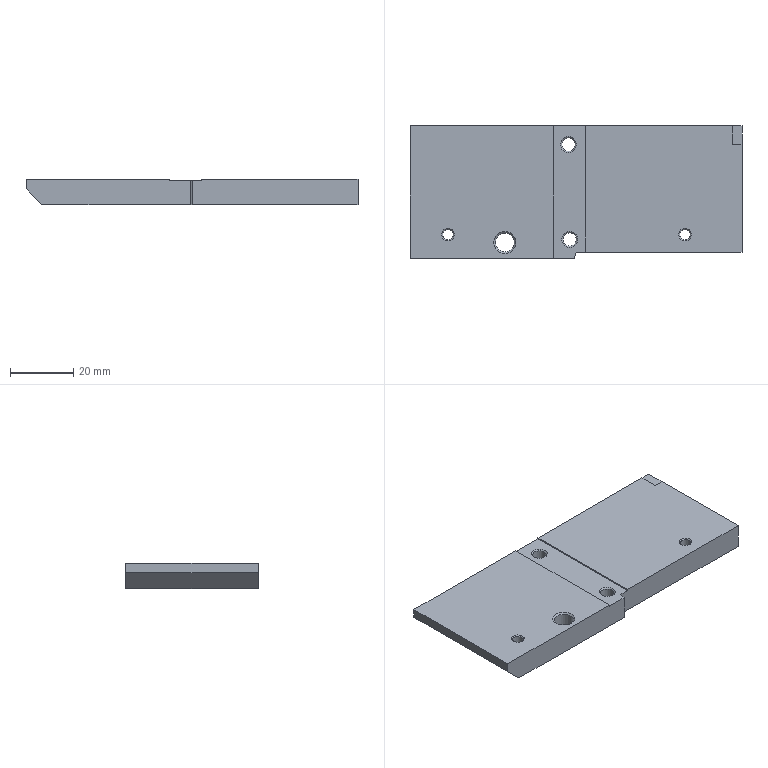Part | 2 solids | 51 faces | box 105 x 42 x 8 mm | volume 32745 mm3 | plane 21 | cone 20 | cylinder 10 | commonest cylinder face diameters 2.5 x4 4.2 x3 3.3 x2 6 x1
STEP:
#1=CARTESIAN_POINT('',(-22.5,21.,-6.2));
#2=VERTEX_POINT('',#1);
#3=CARTESIAN_POINT('',(-22.5,21.,-3.7));
#4=DIRECTION('',(0.,-1.,0.));
#5=DIRECTION('',(0.,0.,-1.));
#6=AXIS2_PLACEMENT_3D('',#3,#4,#5);
#7=CIRCLE('',#6,2.5);
#8=EDGE_CURVE('',#2,#2,#7,.T.);
#9=ORIENTED_EDGE('',*,*,#8,.T.);
#10=EDGE_LOOP('',(#9));
#11=FACE_BOUND('',#10,.T.);
#12=CARTESIAN_POINT('',(36.5,21.,-6.));
#13=VERTEX_POINT('',#12);
#14=CARTESIAN_POINT('',(36.5,21.,-4.5));
#15=DIRECTION('',(0.,-1.,0.));
#16=DIRECTION('',(0.,0.,-1.));
#17=AXIS2_PLACEMENT_3D('',#14,#15,#16);
#18=CIRCLE('',#17,1.5);
#19=EDGE_CURVE('',#13,#13,#18,.T.);
#20=ORIENTED_EDGE('',*,*,#19,.T.);
#21=EDGE_LOOP('',(#20));
#22=FACE_BOUND('',#21,.T.);
#23=CARTESIAN_POINT('',(8.5,21.,-6.));
#24=VERTEX_POINT('',#23);
#25=CARTESIAN_POINT('',(8.5,21.,-4.5));
#26=DIRECTION('',(0.,-1.,0.));
#27=DIRECTION('',(0.,0.,-1.));
#28=AXIS2_PLACEMENT_3D('',#25,#26,#27);
#29=CIRCLE('',#28,1.5);
#30=EDGE_CURVE('',#24,#24,#29,.T.);
#31=ORIENTED_EDGE('',*,*,#30,.T.);
#32=EDGE_LOOP('',(#31));
#33=FACE_BOUND('',#32,.T.);
#34=CARTESIAN_POINT('',(-36.5,21.,-5.2));
#35=VERTEX_POINT('',#34);
#36=CARTESIAN_POINT('',(-36.5,21.,-3.7));
#37=DIRECTION('',(0.,-1.,0.));
#38=DIRECTION('',(0.,0.,-1.));
#39=AXIS2_PLACEMENT_3D('',#36,#37,#38);
#40=CIRCLE('',#39,1.5);
#41=EDGE_CURVE('',#35,#35,#40,.T.);
#42=ORIENTED_EDGE('',*,*,#41,.T.);
#43=EDGE_LOOP('',(#42));
#44=FACE_BOUND('',#43,.T.);
#45=CARTESIAN_POINT('',(-44.5,21.,-5.2));
#46=VERTEX_POINT('',#45);
#47=CARTESIAN_POINT('',(-44.5,21.,-3.7));
#48=DIRECTION('',(0.,-1.,0.));
#49=DIRECTION('',(0.,0.,-1.));
#50=AXIS2_PLACEMENT_3D('',#47,#48,#49);
#51=CIRCLE('',#50,1.5);
#52=EDGE_CURVE('',#46,#46,#51,.T.);
#53=ORIENTED_EDGE('',*,*,#52,.T.);
#54=EDGE_LOOP('',(#53));
#55=FACE_BOUND('',#54,.T.);
#56=CARTESIAN_POINT('',(-47.5,21.,-8.));
#57=VERTEX_POINT('',#56);
#58=CARTESIAN_POINT('',(49.5,21.,-8.));
#59=VERTEX_POINT('',#58);
#60=CARTESIAN_POINT('',(-52.5,21.,-8.));
#61=DIRECTION('',(1.,0.,0.));
#62=VECTOR('',#61,1000.);
#63=LINE('',#60,#62);
#64=EDGE_CURVE('',#57,#59,#63,.T.);
#65=ORIENTED_EDGE('',*,*,#64,.F.);
#66=CARTESIAN_POINT('',(-52.5,21.,-3.));
#67=VERTEX_POINT('',#66);
#68=CARTESIAN_POINT('',(-47.5,21.,-8.));
#69=DIRECTION('',(-0.7071,0.,0.7071));
#70=VECTOR('',#69,1000.);
#71=LINE('',#68,#70);
#72=EDGE_CURVE('',#57,#67,#71,.T.);
#73=ORIENTED_EDGE('',*,*,#72,.T.);
#74=CARTESIAN_POINT('',(-52.5,21.,0.));
#75=VERTEX_POINT('',#74);
#76=CARTESIAN_POINT('',(-52.5,21.,-8.));
#77=DIRECTION('',(0.,0.,1.));
#78=VECTOR('',#77,1000.);
#79=LINE('',#76,#78);
#80=EDGE_CURVE('',#67,#75,#79,.T.);
#81=ORIENTED_EDGE('',*,*,#80,.T.);
#82=CARTESIAN_POINT('',(-7.,21.,0.));
#83=VERTEX_POINT('',#82);
#84=CARTESIAN_POINT('',(-52.5,21.,0.));
#85=DIRECTION('',(1.,0.,0.));
#86=VECTOR('',#85,1000.);
#87=LINE('',#84,#86);
#88=EDGE_CURVE('',#75,#83,#87,.T.);
#89=ORIENTED_EDGE('',*,*,#88,.T.);
#90=CARTESIAN_POINT('',(-7.,21.,-0.4));
#91=VERTEX_POINT('',#90);
#92=CARTESIAN_POINT('',(-7.,21.,-0.4));
#93=DIRECTION('',(0.,0.,1.));
#94=VECTOR('',#93,1000.);
#95=LINE('',#92,#94);
#96=EDGE_CURVE('',#91,#83,#95,.T.);
#97=ORIENTED_EDGE('',*,*,#96,.F.);
#98=CARTESIAN_POINT('',(3.,21.,-0.4));
#99=VERTEX_POINT('',#98);
#100=CARTESIAN_POINT('',(3.,21.,-0.4));
#101=DIRECTION('',(-1.,0.,0.));
#102=VECTOR('',#101,1000.);
#103=LINE('',#100,#102);
#104=EDGE_CURVE('',#99,#91,#103,.T.);
#105=ORIENTED_EDGE('',*,*,#104,.F.);
#106=CARTESIAN_POINT('',(3.,21.,0.));
#107=VERTEX_POINT('',#106);
#108=CARTESIAN_POINT('',(3.,21.,0.));
#109=DIRECTION('',(0.,0.,-1.));
#110=VECTOR('',#109,1000.);
#111=LINE('',#108,#110);
#112=EDGE_CURVE('',#107,#99,#111,.T.);
#113=ORIENTED_EDGE('',*,*,#112,.F.);
#114=CARTESIAN_POINT('',(49.5,21.,0.));
#115=VERTEX_POINT('',#114);
#116=CARTESIAN_POINT('',(-52.5,21.,0.));
#117=DIRECTION('',(1.,0.,0.));
#118=VECTOR('',#117,1000.);
#119=LINE('',#116,#118);
#120=EDGE_CURVE('',#107,#115,#119,.T.);
#121=ORIENTED_EDGE('',*,*,#120,.T.);
#122=CARTESIAN_POINT('',(49.5,21.,-8.));
#123=DIRECTION('',(0.,0.,1.));
#124=VECTOR('',#123,1000.);
#125=LINE('',#122,#124);
#126=EDGE_CURVE('',#59,#115,#125,.T.);
#127=ORIENTED_EDGE('',*,*,#126,.F.);
#128=EDGE_LOOP('',(#65,#73,#81,#89,#97,#105,#113,#121,#127));
#129=FACE_BOUND('',#128,.T.);
#130=CARTESIAN_POINT('',(-52.5,21.,-8.));
#131=DIRECTION('',(0.,-1.,0.));
#132=DIRECTION('',(0.,0.,1.));
#133=AXIS2_PLACEMENT_3D('',#130,#131,#132);
#134=PLANE('',#133);
#135=ADVANCED_FACE('',(#11,#22,#33,#44,#55,#129),#134,.F.);
#136=CARTESIAN_POINT('',(34.5,-11.5,0.));
#137=VERTEX_POINT('',#136);
#138=CARTESIAN_POINT('',(34.5,-13.5,0.));
#139=DIRECTION('',(0.,0.,-1.));
#140=DIRECTION('',(0.,1.,0.));
#141=AXIS2_PLACEMENT_3D('',#138,#139,#140);
#142=CIRCLE('',#141,2.);
#143=EDGE_CURVE('',#137,#137,#142,.T.);
#144=ORIENTED_EDGE('',*,*,#143,.T.);
#145=EDGE_LOOP('',(#144));
#146=FACE_BOUND('',#145,.T.);
#147=CARTESIAN_POINT('',(3.,-19.,0.));
#148=VERTEX_POINT('',#147);
#149=CARTESIAN_POINT('',(3.,-76.,0.));
#150=DIRECTION('',(0.,1.,0.));
#151=VECTOR('',#150,1000.);
#152=LINE('',#149,#151);
#153=EDGE_CURVE('',#148,#107,#152,.T.);
#154=ORIENTED_EDGE('',*,*,#153,.F.);
#155=CARTESIAN_POINT('',(52.5,-19.,0.));
#156=VERTEX_POINT('',#155);
#157=CARTESIAN_POINT('',(52.5,-19.,0.));
#158=DIRECTION('',(-1.,0.,0.));
#159=VECTOR('',#158,1000.);
#160=LINE('',#157,#159);
#161=EDGE_CURVE('',#156,#148,#160,.T.);
#162=ORIENTED_EDGE('',*,*,#161,.F.);
#163=CARTESIAN_POINT('',(52.5,15.,0.));
#164=VERTEX_POINT('',#163);
#165=CARTESIAN_POINT('',(52.5,15.,0.));
#166=DIRECTION('',(0.,-1.,0.));
#167=VECTOR('',#166,1000.);
#168=LINE('',#165,#167);
#169=EDGE_CURVE('',#164,#156,#168,.T.);
#170=ORIENTED_EDGE('',*,*,#169,.F.);
#171=CARTESIAN_POINT('',(49.5,15.,0.));
#172=VERTEX_POINT('',#171);
#173=CARTESIAN_POINT('',(49.5,15.,0.));
#174=DIRECTION('',(1.,0.,0.));
#175=VECTOR('',#174,1000.);
#176=LINE('',#173,#175);
#177=EDGE_CURVE('',#172,#164,#176,.T.);
#178=ORIENTED_EDGE('',*,*,#177,.F.);
#179=CARTESIAN_POINT('',(49.5,21.,0.));
#180=DIRECTION('',(0.,-1.,0.));
#181=VECTOR('',#180,1000.);
#182=LINE('',#179,#181);
#183=EDGE_CURVE('',#115,#172,#182,.T.);
#184=ORIENTED_EDGE('',*,*,#183,.F.);
#185=ORIENTED_EDGE('',*,*,#120,.F.);
#186=EDGE_LOOP('',(#154,#162,#170,#178,#184,#185));
#187=FACE_BOUND('',#186,.T.);
#188=CARTESIAN_POINT('',(-52.5,21.,0.));
#189=DIRECTION('',(0.,0.,-1.));
#190=DIRECTION('',(0.,-1.,0.));
#191=AXIS2_PLACEMENT_3D('',#188,#189,#190);
#192=PLANE('',#191);
#193=ADVANCED_FACE('',(#146,#187),#192,.F.);
#194=CARTESIAN_POINT('',(-52.5,-21.,-3.));
#195=VERTEX_POINT('',#194);
#196=CARTESIAN_POINT('',(-52.5,-21.,0.));
#197=VERTEX_POINT('',#196);
#198=CARTESIAN_POINT('',(-52.5,-21.,-8.));
#199=DIRECTION('',(0.,0.,1.));
#200=VECTOR('',#199,1000.);
#201=LINE('',#198,#200);
#202=EDGE_CURVE('',#195,#197,#201,.T.);
#203=ORIENTED_EDGE('',*,*,#202,.F.);
#204=CARTESIAN_POINT('',(-47.5,-21.,-8.));
#205=VERTEX_POINT('',#204);
#206=CARTESIAN_POINT('',(-47.5,-21.,-8.));
#207=DIRECTION('',(0.7071,0.,-0.7071));
#208=VECTOR('',#207,1000.);
#209=LINE('',#206,#208);
#210=EDGE_CURVE('',#195,#205,#209,.T.);
#211=ORIENTED_EDGE('',*,*,#210,.T.);
#212=CARTESIAN_POINT('',(-0.5,-21.,-8.));
#213=VERTEX_POINT('',#212);
#214=CARTESIAN_POINT('',(-0.5,-21.,-8.));
#215=DIRECTION('',(-1.,0.,0.));
#216=VECTOR('',#215,1000.);
#217=LINE('',#214,#216);
#218=EDGE_CURVE('',#213,#205,#217,.T.);
#219=ORIENTED_EDGE('',*,*,#218,.F.);
#220=CARTESIAN_POINT('',(-0.5,-21.,-0.4));
#221=VERTEX_POINT('',#220);
#222=CARTESIAN_POINT('',(-0.5,-21.,-8.));
#223=DIRECTION('',(0.,0.,1.));
#224=VECTOR('',#223,1000.);
#225=LINE('',#222,#224);
#226=EDGE_CURVE('',#213,#221,#225,.T.);
#227=ORIENTED_EDGE('',*,*,#226,.T.);
#228=CARTESIAN_POINT('',(-7.,-21.,-0.4));
#229=VERTEX_POINT('',#228);
#230=CARTESIAN_POINT('',(-0.5,-21.,-0.4));
#231=DIRECTION('',(-1.,0.,0.));
#232=VECTOR('',#231,1000.);
#233=LINE('',#230,#232);
#234=EDGE_CURVE('',#221,#229,#233,.T.);
#235=ORIENTED_EDGE('',*,*,#234,.T.);
#236=CARTESIAN_POINT('',(-7.,-21.,0.));
#237=VERTEX_POINT('',#236);
#238=CARTESIAN_POINT('',(-7.,-21.,-8.));
#239=DIRECTION('',(0.,0.,1.));
#240=VECTOR('',#239,1000.);
#241=LINE('',#238,#240);
#242=EDGE_CURVE('',#229,#237,#241,.T.);
#243=ORIENTED_EDGE('',*,*,#242,.T.);
#244=CARTESIAN_POINT('',(-0.5,-21.,0.));
#245=DIRECTION('',(-1.,0.,0.));
#246=VECTOR('',#245,1000.);
#247=LINE('',#244,#246);
#248=EDGE_CURVE('',#237,#197,#247,.T.);
#249=ORIENTED_EDGE('',*,*,#248,.T.);
#250=EDGE_LOOP('',(#203,#211,#219,#227,#235,#243,#249));
#251=FACE_BOUND('',#250,.T.);
#252=CARTESIAN_POINT('',(-0.5,-21.,-8.));
#253=DIRECTION('',(0.,1.,0.));
#254=DIRECTION('',(0.,0.,-1.));
#255=AXIS2_PLACEMENT_3D('',#252,#253,#254);
#256=PLANE('',#255);
#257=ADVANCED_FACE('',(#251),#256,.F.);
#258=ORIENTED_EDGE('',*,*,#80,.F.);
#259=CARTESIAN_POINT('',(-52.5,-21.,-3.));
#260=DIRECTION('',(0.,-1.,0.));
#261=VECTOR('',#260,1000.);
#262=LINE('',#259,#261);
#263=EDGE_CURVE('',#67,#195,#262,.T.);
#264=ORIENTED_EDGE('',*,*,#263,.T.);
#265=ORIENTED_EDGE('',*,*,#202,.T.);
#266=CARTESIAN_POINT('',(-52.5,-21.,0.));
#267=DIRECTION('',(0.,1.,0.));
#268=VECTOR('',#267,1000.);
#269=LINE('',#266,#268);
#270=EDGE_CURVE('',#197,#75,#269,.T.);
#271=ORIENTED_EDGE('',*,*,#270,.T.);
#272=EDGE_LOOP('',(#258,#264,#265,#271));
#273=FACE_BOUND('',#272,.T.);
#274=CARTESIAN_POINT('',(-52.5,-21.,-8.));
#275=DIRECTION('',(1.,0.,0.));
#276=DIRECTION('',(0.,1.,0.));
#277=AXIS2_PLACEMENT_3D('',#274,#275,#276);
#278=PLANE('',#277);
#279=ADVANCED_FACE('',(#273),#278,.F.);
#280=ORIENTED_EDGE('',*,*,#183,.T.);
#281=CARTESIAN_POINT('',(49.5,15.,-8.));
#282=VERTEX_POINT('',#281);
#283=CARTESIAN_POINT('',(49.5,15.,-8.));
#284=DIRECTION('',(0.,0.,1.));
#285=VECTOR('',#284,1000.);
#286=LINE('',#283,#285);
#287=EDGE_CURVE('',#282,#172,#286,.T.);
#288=ORIENTED_EDGE('',*,*,#287,.F.);
#289=CARTESIAN_POINT('',(49.5,21.,-8.));
#290=DIRECTION('',(0.,-1.,0.));
#291=VECTOR('',#290,1000.);
#292=LINE('',#289,#291);
#293=EDGE_CURVE('',#59,#282,#292,.T.);
#294=ORIENTED_EDGE('',*,*,#293,.F.);
#295=ORIENTED_EDGE('',*,*,#126,.T.);
#296=EDGE_LOOP('',(#280,#288,#294,#295));
#297=FACE_BOUND('',#296,.T.);
#298=CARTESIAN_POINT('',(49.5,21.,-8.));
#299=DIRECTION('',(-1.,0.,0.));
#300=DIRECTION('',(0.,-1.,0.));
#301=AXIS2_PLACEMENT_3D('',#298,#299,#300);
#302=PLANE('',#301);
#303=ADVANCED_FACE('',(#297),#302,.F.);
#304=ORIENTED_EDGE('',*,*,#177,.T.);
#305=CARTESIAN_POINT('',(52.5,15.,-8.));
#306=VERTEX_POINT('',#305);
#307=CARTESIAN_POINT('',(52.5,15.,-8.));
#308=DIRECTION('',(0.,0.,1.));
#309=VECTOR('',#308,1000.);
#310=LINE('',#307,#309);
#311=EDGE_CURVE('',#306,#164,#310,.T.);
#312=ORIENTED_EDGE('',*,*,#311,.F.);
#313=CARTESIAN_POINT('',(49.5,15.,-8.));
#314=DIRECTION('',(1.,0.,0.));
#315=VECTOR('',#314,1000.);
#316=LINE('',#313,#315);
#317=EDGE_CURVE('',#282,#306,#316,.T.);
#318=ORIENTED_EDGE('',*,*,#317,.F.);
#319=ORIENTED_EDGE('',*,*,#287,.T.);
#320=EDGE_LOOP('',(#304,#312,#318,#319));
#321=FACE_BOUND('',#320,.T.);
#322=CARTESIAN_POINT('',(49.5,15.,-8.));
#323=DIRECTION('',(0.,-1.,0.));
#324=DIRECTION('',(0.,0.,1.));
#325=AXIS2_PLACEMENT_3D('',#322,#323,#324);
#326=PLANE('',#325);
#327=ADVANCED_FACE('',(#321),#326,.F.);
#328=ORIENTED_EDGE('',*,*,#169,.T.);
#329=CARTESIAN_POINT('',(52.5,-19.,-8.));
#330=VERTEX_POINT('',#329);
#331=CARTESIAN_POINT('',(52.5,-19.,-8.));
#332=DIRECTION('',(0.,0.,1.));
#333=VECTOR('',#332,1000.);
#334=LINE('',#331,#333);
#335=EDGE_CURVE('',#330,#156,#334,.T.);
#336=ORIENTED_EDGE('',*,*,#335,.F.);
#337=CARTESIAN_POINT('',(52.5,15.,-8.));
#338=DIRECTION('',(0.,-1.,0.));
#339=VECTOR('',#338,1000.);
#340=LINE('',#337,#339);
#341=EDGE_CURVE('',#306,#330,#340,.T.);
#342=ORIENTED_EDGE('',*,*,#341,.F.);
#343=ORIENTED_EDGE('',*,*,#311,.T.);
#344=EDGE_LOOP('',(#328,#336,#342,#343));
#345=FACE_BOUND('',#344,.T.);
#346=CARTESIAN_POINT('',(52.5,15.,-8.));
#347=DIRECTION('',(-1.,0.,0.));
#348=DIRECTION('',(0.,-1.,0.));
#349=AXIS2_PLACEMENT_3D('',#346,#347,#348);
#350=PLANE('',#349);
#351=ADVANCED_FACE('',(#345),#350,.F.);
#352=CARTESIAN_POINT('',(3.,-19.,-0.4));
#353=VERTEX_POINT('',#352);
#354=CARTESIAN_POINT('',(3.,-19.,-8.));
#355=DIRECTION('',(0.,0.,-1.));
#356=VECTOR('',#355,1000.);
#357=LINE('',#354,#356);
#358=EDGE_CURVE('',#148,#353,#357,.T.);
#359=ORIENTED_EDGE('',*,*,#358,.T.);
#360=CARTESIAN_POINT('',(0.0359,-19.,-0.4));
#361=VERTEX_POINT('',#360);
#362=CARTESIAN_POINT('',(52.5,-19.,-0.4));
#363=DIRECTION('',(-1.,0.,0.));
#364=VECTOR('',#363,1000.);
#365=LINE('',#362,#364);
#366=EDGE_CURVE('',#353,#361,#365,.T.);
#367=ORIENTED_EDGE('',*,*,#366,.T.);
#368=CARTESIAN_POINT('',(0.0359,-19.,-8.));
#369=VERTEX_POINT('',#368);
#370=CARTESIAN_POINT('',(0.0359,-19.,-8.));
#371=DIRECTION('',(0.,0.,1.));
#372=VECTOR('',#371,1000.);
#373=LINE('',#370,#372);
#374=EDGE_CURVE('',#369,#361,#373,.T.);
#375=ORIENTED_EDGE('',*,*,#374,.F.);
#376=CARTESIAN_POINT('',(52.5,-19.,-8.));
#377=DIRECTION('',(-1.,0.,0.));
#378=VECTOR('',#377,1000.);
#379=LINE('',#376,#378);
#380=EDGE_CURVE('',#330,#369,#379,.T.);
#381=ORIENTED_EDGE('',*,*,#380,.F.);
#382=ORIENTED_EDGE('',*,*,#335,.T.);
#383=ORIENTED_EDGE('',*,*,#161,.T.);
#384=EDGE_LOOP('',(#359,#367,#375,#381,#382,#383));
#385=FACE_BOUND('',#384,.T.);
#386=CARTESIAN_POINT('',(52.5,-19.,-8.));
#387=DIRECTION('',(0.,1.,0.));
#388=DIRECTION('',(0.,0.,-1.));
#389=AXIS2_PLACEMENT_3D('',#386,#387,#388);
#390=PLANE('',#389);
#391=ADVANCED_FACE('',(#385),#390,.F.);
#392=ORIENTED_EDGE('',*,*,#374,.T.);
#393=CARTESIAN_POINT('',(0.0359,-19.,-0.4));
#394=DIRECTION('',(-0.2588,-0.9659,0.));
#395=VECTOR('',#394,1000.);
#396=LINE('',#393,#395);
#397=EDGE_CURVE('',#361,#221,#396,.T.);
#398=ORIENTED_EDGE('',*,*,#397,.T.);
#399=ORIENTED_EDGE('',*,*,#226,.F.);
#400=CARTESIAN_POINT('',(0.0359,-19.,-8.));
#401=DIRECTION('',(-0.2588,-0.9659,0.));
#402=VECTOR('',#401,1000.);
#403=LINE('',#400,#402);
#404=EDGE_CURVE('',#369,#213,#403,.T.);
#405=ORIENTED_EDGE('',*,*,#404,.F.);
#406=EDGE_LOOP('',(#392,#398,#399,#405));
#407=FACE_BOUND('',#406,.T.);
#408=CARTESIAN_POINT('',(0.0359,-19.,-8.));
#409=DIRECTION('',(-0.9659,0.2588,0.));
#410=DIRECTION('',(-0.2588,-0.9659,0.));
#411=AXIS2_PLACEMENT_3D('',#408,#409,#410);
#412=PLANE('',#411);
#413=ADVANCED_FACE('',(#407),#412,.F.);
#414=CARTESIAN_POINT('',(-22.5,-12.5,-8.));
#415=VERTEX_POINT('',#414);
#416=CARTESIAN_POINT('',(-22.5,-16.,-8.));
#417=DIRECTION('',(0.,0.,-1.));
#418=DIRECTION('',(0.,1.,0.));
#419=AXIS2_PLACEMENT_3D('',#416,#417,#418);
#420=CIRCLE('',#419,3.5);
#421=EDGE_CURVE('',#415,#415,#420,.T.);
#422=ORIENTED_EDGE('',*,*,#421,.F.);
#423=EDGE_LOOP('',(#422));
#424=FACE_BOUND('',#423,.T.);
#425=CARTESIAN_POINT('',(34.5,-11.5,-8.));
#426=VERTEX_POINT('',#425);
#427=CARTESIAN_POINT('',(34.5,-13.5,-8.));
#428=DIRECTION('',(0.,0.,-1.));
#429=DIRECTION('',(0.,1.,0.));
#430=AXIS2_PLACEMENT_3D('',#427,#428,#429);
#431=CIRCLE('',#430,2.);
#432=EDGE_CURVE('',#426,#426,#431,.T.);
#433=ORIENTED_EDGE('',*,*,#432,.F.);
#434=EDGE_LOOP('',(#433));
#435=FACE_BOUND('',#434,.T.);
#436=CARTESIAN_POINT('',(-40.5,-11.5,-8.));
#437=VERTEX_POINT('',#436);
#438=CARTESIAN_POINT('',(-40.5,-13.5,-8.));
#439=DIRECTION('',(0.,0.,-1.));
#440=DIRECTION('',(0.,1.,0.));
#441=AXIS2_PLACEMENT_3D('',#438,#439,#440);
#442=CIRCLE('',#441,2.);
#443=EDGE_CURVE('',#437,#437,#442,.T.);
#444=ORIENTED_EDGE('',*,*,#443,.F.);
#445=EDGE_LOOP('',(#444));
#446=FACE_BOUND('',#445,.T.);
#447=CARTESIAN_POINT('',(-2.,-12.5,-8.));
#448=VERTEX_POINT('',#447);
#449=CARTESIAN_POINT('',(-2.,-15.,-8.));
#450=DIRECTION('',(0.,0.,-1.));
#451=DIRECTION('',(0.,1.,0.));
#452=AXIS2_PLACEMENT_3D('',#449,#450,#451);
#453=CIRCLE('',#452,2.5);
#454=EDGE_CURVE('',#448,#448,#453,.T.);
#455=ORIENTED_EDGE('',*,*,#454,.F.);
#456=EDGE_LOOP('',(#455));
#457=FACE_BOUND('',#456,.T.);
#458=CARTESIAN_POINT('',(-2.382,17.498,-8.));
#459=VERTEX_POINT('',#458);
#460=CARTESIAN_POINT('',(-2.382,14.998,-8.));
#461=DIRECTION('',(0.,0.,-1.));
#462=DIRECTION('',(0.,1.,0.));
#463=AXIS2_PLACEMENT_3D('',#460,#461,#462);
#464=CIRCLE('',#463,2.5);
#465=EDGE_CURVE('',#459,#459,#464,.T.);
#466=ORIENTED_EDGE('',*,*,#465,.F.);
#467=EDGE_LOOP('',(#466));
#468=FACE_BOUND('',#467,.T.);
#469=ORIENTED_EDGE('',*,*,#218,.T.);
#470=CARTESIAN_POINT('',(-47.5,21.,-8.));
#471=DIRECTION('',(0.,1.,0.));
#472=VECTOR('',#471,1000.);
#473=LINE('',#470,#472);
#474=EDGE_CURVE('',#205,#57,#473,.T.);
#475=ORIENTED_EDGE('',*,*,#474,.T.);
#476=ORIENTED_EDGE('',*,*,#64,.T.);
#477=ORIENTED_EDGE('',*,*,#293,.T.);
#478=ORIENTED_EDGE('',*,*,#317,.T.);
#479=ORIENTED_EDGE('',*,*,#341,.T.);
#480=ORIENTED_EDGE('',*,*,#380,.T.);
#481=ORIENTED_EDGE('',*,*,#404,.T.);
#482=EDGE_LOOP('',(#469,#475,#476,#477,#478,#479,#480,#481));
#483=FACE_BOUND('',#482,.T.);
#484=CARTESIAN_POINT('',(-52.5,21.,-8.));
#485=DIRECTION('',(0.,0.,-1.));
#486=DIRECTION('',(0.,-1.,0.));
#487=AXIS2_PLACEMENT_3D('',#484,#485,#486);
#488=PLANE('',#487);
#489=ADVANCED_FACE('',(#424,#435,#446,#457,#468,#483),#488,.T.);
#490=CARTESIAN_POINT('',(-22.5,-12.5,0.));
#491=VERTEX_POINT('',#490);
#492=CARTESIAN_POINT('',(-22.5,-16.,0.));
#493=DIRECTION('',(0.,0.,-1.));
#494=DIRECTION('',(0.,1.,0.));
#495=AXIS2_PLACEMENT_3D('',#492,#493,#494);
#496=CIRCLE('',#495,3.5);
#497=EDGE_CURVE('',#491,#491,#496,.T.);
#498=ORIENTED_EDGE('',*,*,#497,.T.);
#499=EDGE_LOOP('',(#498));
#500=FACE_BOUND('',#499,.T.);
#501=CARTESIAN_POINT('',(-40.5,-11.5,0.));
#502=VERTEX_POINT('',#501);
#503=CARTESIAN_POINT('',(-40.5,-13.5,0.));
#504=DIRECTION('',(0.,0.,-1.));
#505=DIRECTION('',(0.,1.,0.));
#506=AXIS2_PLACEMENT_3D('',#503,#504,#505);
#507=CIRCLE('',#506,2.);
#508=EDGE_CURVE('',#502,#502,#507,.T.);
#509=ORIENTED_EDGE('',*,*,#508,.T.);
#510=EDGE_LOOP('',(#509));
#511=FACE_BOUND('',#510,.T.);
#512=ORIENTED_EDGE('',*,*,#248,.F.);
#513=CARTESIAN_POINT('',(-7.,-76.,0.));
#514=DIRECTION('',(0.,1.,0.));
#515=VECTOR('',#514,1000.);
#516=LINE('',#513,#515);
#517=EDGE_CURVE('',#237,#83,#516,.T.);
#518=ORIENTED_EDGE('',*,*,#517,.T.);
#519=ORIENTED_EDGE('',*,*,#88,.F.);
#520=ORIENTED_EDGE('',*,*,#270,.F.);
#521=EDGE_LOOP('',(#512,#518,#519,#520));
#522=FACE_BOUND('',#521,.T.);
#523=CARTESIAN_POINT('',(-52.5,21.,0.));
#524=DIRECTION('',(0.,0.,-1.));
#525=DIRECTION('',(0.,-1.,0.));
#526=AXIS2_PLACEMENT_3D('',#523,#524,#525);
#527=PLANE('',#526);
#528=ADVANCED_FACE('',(#500,#511,#522),#527,.F.);
#529=CARTESIAN_POINT('',(-7.,-76.,-0.4));
#530=DIRECTION('',(0.,-1.,0.));
#531=VECTOR('',#530,1000.);
#532=LINE('',#529,#531);
#533=EDGE_CURVE('',#91,#229,#532,.T.);
#534=ORIENTED_EDGE('',*,*,#533,.F.);
#535=ORIENTED_EDGE('',*,*,#96,.T.);
#536=ORIENTED_EDGE('',*,*,#517,.F.);
#537=ORIENTED_EDGE('',*,*,#242,.F.);
#538=EDGE_LOOP('',(#534,#535,#536,#537));
#539=FACE_BOUND('',#538,.T.);
#540=CARTESIAN_POINT('',(-7.,-76.,-0.4));
#541=DIRECTION('',(-1.,0.,0.));
#542=DIRECTION('',(0.,-1.,0.));
#543=AXIS2_PLACEMENT_3D('',#540,#541,#542);
#544=PLANE('',#543);
#545=ADVANCED_FACE('',(#539),#544,.F.);
#546=CARTESIAN_POINT('',(-2.,-12.5,-0.4));
#547=VERTEX_POINT('',#546);
#548=CARTESIAN_POINT('',(-2.,-15.,-0.4));
#549=DIRECTION('',(0.,0.,-1.));
#550=DIRECTION('',(0.,1.,0.));
#551=AXIS2_PLACEMENT_3D('',#548,#549,#550);
#552=CIRCLE('',#551,2.5);
#553=EDGE_CURVE('',#547,#547,#552,.T.);
#554=ORIENTED_EDGE('',*,*,#553,.T.);
#555=EDGE_LOOP('',(#554));
#556=FACE_BOUND('',#555,.T.);
#557=CARTESIAN_POINT('',(-2.382,17.498,-0.4));
#558=VERTEX_POINT('',#557);
#559=CARTESIAN_POINT('',(-2.382,14.998,-0.4));
#560=DIRECTION('',(0.,0.,-1.));
#561=DIRECTION('',(0.,1.,0.));
#562=AXIS2_PLACEMENT_3D('',#559,#560,#561);
#563=CIRCLE('',#562,2.5);
#564=EDGE_CURVE('',#558,#558,#563,.T.);
#565=ORIENTED_EDGE('',*,*,#564,.T.);
#566=EDGE_LOOP('',(#565));
#567=FACE_BOUND('',#566,.T.);
#568=ORIENTED_EDGE('',*,*,#397,.F.);
#569=ORIENTED_EDGE('',*,*,#366,.F.);
#570=CARTESIAN_POINT('',(3.,-76.,-0.4));
#571=DIRECTION('',(0.,-1.,0.));
#572=VECTOR('',#571,1000.);
#573=LINE('',#570,#572);
#574=EDGE_CURVE('',#99,#353,#573,.T.);
#575=ORIENTED_EDGE('',*,*,#574,.F.);
#576=ORIENTED_EDGE('',*,*,#104,.T.);
#577=ORIENTED_EDGE('',*,*,#533,.T.);
#578=ORIENTED_EDGE('',*,*,#234,.F.);
#579=EDGE_LOOP('',(#568,#569,#575,#576,#577,#578));
#580=FACE_BOUND('',#579,.T.);
#581=CARTESIAN_POINT('',(3.,-76.,-0.4));
#582=DIRECTION('',(0.,0.,-1.));
#583=DIRECTION('',(0.,-1.,0.));
#584=AXIS2_PLACEMENT_3D('',#581,#582,#583);
#585=PLANE('',#584);
#586=ADVANCED_FACE('',(#556,#567,#580),#585,.F.);
#587=ORIENTED_EDGE('',*,*,#153,.T.);
#588=ORIENTED_EDGE('',*,*,#112,.T.);
#589=ORIENTED_EDGE('',*,*,#574,.T.);
#590=ORIENTED_EDGE('',*,*,#358,.F.);
#591=EDGE_LOOP('',(#587,#588,#589,#590));
#592=FACE_BOUND('',#591,.T.);
#593=CARTESIAN_POINT('',(3.,-76.,0.));
#594=DIRECTION('',(1.,0.,0.));
#595=DIRECTION('',(0.,1.,0.));
#596=AXIS2_PLACEMENT_3D('',#593,#594,#595);
#597=PLANE('',#596);
#598=ADVANCED_FACE('',(#592),#597,.F.);
#599=CARTESIAN_POINT('',(-2.382,17.098,-7.6));
#600=VERTEX_POINT('',#599);
#601=CARTESIAN_POINT('',(-2.382,14.998,-7.6));
#602=DIRECTION('',(0.,0.,-1.));
#603=DIRECTION('',(0.,1.,0.));
#604=AXIS2_PLACEMENT_3D('',#601,#602,#603);
#605=CIRCLE('',#604,2.1);
#606=EDGE_CURVE('',#600,#600,#605,.T.);
#607=ORIENTED_EDGE('',*,*,#606,.T.);
#608=EDGE_LOOP('',(#607));
#609=FACE_BOUND('',#608,.T.);
#610=CARTESIAN_POINT('',(-2.382,12.898,-0.8));
#611=VERTEX_POINT('',#610);
#612=CARTESIAN_POINT('',(-2.382,14.998,-0.8));
#613=DIRECTION('',(0.,0.,1.));
#614=DIRECTION('',(0.,-1.,0.));
#615=AXIS2_PLACEMENT_3D('',#612,#613,#614);
#616=CIRCLE('',#615,2.1);
#617=EDGE_CURVE('',#611,#611,#616,.T.);
#618=ORIENTED_EDGE('',*,*,#617,.T.);
#619=EDGE_LOOP('',(#618));
#620=FACE_BOUND('',#619,.T.);
#621=CARTESIAN_POINT('',(-2.382,14.998,0.));
#622=DIRECTION('',(0.,0.,-1.));
#623=DIRECTION('',(0.,-1.,0.));
#624=AXIS2_PLACEMENT_3D('',#621,#622,#623);
#625=CYLINDRICAL_SURFACE('',#624,2.1);
#626=ADVANCED_FACE('',(#609,#620),#625,.F.);
#627=ORIENTED_EDGE('',*,*,#564,.F.);
#628=EDGE_LOOP('',(#627));
#629=FACE_BOUND('',#628,.T.);
#630=ORIENTED_EDGE('',*,*,#617,.F.);
#631=EDGE_LOOP('',(#630));
#632=FACE_BOUND('',#631,.T.);
#633=CARTESIAN_POINT('',(-2.382,14.998,-2.9));
#634=DIRECTION('',(0.,0.,1.));
#635=DIRECTION('',(1.,0.,0.));
#636=AXIS2_PLACEMENT_3D('',#633,#634,#635);
#637=CONICAL_SURFACE('',#636,0.,0.7854);
#638=ADVANCED_FACE('',(#629,#632),#637,.F.);
#639=ORIENTED_EDGE('',*,*,#465,.T.);
#640=EDGE_LOOP('',(#639));
#641=FACE_BOUND('',#640,.T.);
#642=ORIENTED_EDGE('',*,*,#606,.F.);
#643=EDGE_LOOP('',(#642));
#644=FACE_BOUND('',#643,.T.);
#645=CARTESIAN_POINT('',(-2.382,14.998,-5.5));
#646=DIRECTION('',(0.,0.,-1.));
#647=DIRECTION('',(-1.,0.,0.));
#648=AXIS2_PLACEMENT_3D('',#645,#646,#647);
#649=CONICAL_SURFACE('',#648,0.,0.7854);
#650=ADVANCED_FACE('',(#641,#644),#649,.F.);
#651=CARTESIAN_POINT('',(-2.,-12.9,-7.6));
#652=VERTEX_POINT('',#651);
#653=CARTESIAN_POINT('',(-2.,-15.,-7.6));
#654=DIRECTION('',(0.,0.,-1.));
#655=DIRECTION('',(0.,1.,0.));
#656=AXIS2_PLACEMENT_3D('',#653,#654,#655);
#657=CIRCLE('',#656,2.1);
#658=EDGE_CURVE('',#652,#652,#657,.T.);
#659=ORIENTED_EDGE('',*,*,#658,.T.);
#660=EDGE_LOOP('',(#659));
#661=FACE_BOUND('',#660,.T.);
#662=CARTESIAN_POINT('',(-2.,-17.1,-0.8));
#663=VERTEX_POINT('',#662);
#664=CARTESIAN_POINT('',(-2.,-15.,-0.8));
#665=DIRECTION('',(0.,0.,1.));
#666=DIRECTION('',(0.,-1.,0.));
#667=AXIS2_PLACEMENT_3D('',#664,#665,#666);
#668=CIRCLE('',#667,2.1);
#669=EDGE_CURVE('',#663,#663,#668,.T.);
#670=ORIENTED_EDGE('',*,*,#669,.T.);
#671=EDGE_LOOP('',(#670));
#672=FACE_BOUND('',#671,.T.);
#673=CARTESIAN_POINT('',(-2.,-15.,0.));
#674=DIRECTION('',(0.,0.,-1.));
#675=DIRECTION('',(0.,-1.,0.));
#676=AXIS2_PLACEMENT_3D('',#673,#674,#675);
#677=CYLINDRICAL_SURFACE('',#676,2.1);
#678=ADVANCED_FACE('',(#661,#672),#677,.F.);
#679=ORIENTED_EDGE('',*,*,#553,.F.);
#680=EDGE_LOOP('',(#679));
#681=FACE_BOUND('',#680,.T.);
#682=ORIENTED_EDGE('',*,*,#669,.F.);
#683=EDGE_LOOP('',(#682));
#684=FACE_BOUND('',#683,.T.);
#685=CARTESIAN_POINT('',(-2.,-15.,-2.9));
#686=DIRECTION('',(0.,0.,1.));
#687=DIRECTION('',(1.,0.,0.));
#688=AXIS2_PLACEMENT_3D('',#685,#686,#687);
#689=CONICAL_SURFACE('',#688,0.,0.7854);
#690=ADVANCED_FACE('',(#681,#684),#689,.F.);
#691=ORIENTED_EDGE('',*,*,#454,.T.);
#692=EDGE_LOOP('',(#691));
#693=FACE_BOUND('',#692,.T.);
#694=ORIENTED_EDGE('',*,*,#658,.F.);
#695=EDGE_LOOP('',(#694));
#696=FACE_BOUND('',#695,.T.);
#697=CARTESIAN_POINT('',(-2.,-15.,-5.5));
#698=DIRECTION('',(0.,0.,-1.));
#699=DIRECTION('',(-1.,0.,0.));
#700=AXIS2_PLACEMENT_3D('',#697,#698,#699);
#701=CONICAL_SURFACE('',#700,0.,0.7854);
#702=ADVANCED_FACE('',(#693,#696),#701,.F.);
#703=CARTESIAN_POINT('',(-40.5,-11.85,-7.65));
#704=VERTEX_POINT('',#703);
#705=CARTESIAN_POINT('',(-40.5,-13.5,-7.65));
#706=DIRECTION('',(0.,0.,-1.));
#707=DIRECTION('',(0.,1.,0.));
#708=AXIS2_PLACEMENT_3D('',#705,#706,#707);
#709=CIRCLE('',#708,1.65);
#710=EDGE_CURVE('',#704,#704,#709,.T.);
#711=ORIENTED_EDGE('',*,*,#710,.T.);
#712=EDGE_LOOP('',(#711));
#713=FACE_BOUND('',#712,.T.);
#714=CARTESIAN_POINT('',(-40.5,-15.15,-0.35));
#715=VERTEX_POINT('',#714);
#716=CARTESIAN_POINT('',(-40.5,-13.5,-0.35));
#717=DIRECTION('',(0.,0.,1.));
#718=DIRECTION('',(0.,-1.,0.));
#719=AXIS2_PLACEMENT_3D('',#716,#717,#718);
#720=CIRCLE('',#719,1.65);
#721=EDGE_CURVE('',#715,#715,#720,.T.);
#722=ORIENTED_EDGE('',*,*,#721,.T.);
#723=EDGE_LOOP('',(#722));
#724=FACE_BOUND('',#723,.T.);
#725=CARTESIAN_POINT('',(-40.5,-13.5,0.));
#726=DIRECTION('',(0.,0.,-1.));
#727=DIRECTION('',(0.,-1.,0.));
#728=AXIS2_PLACEMENT_3D('',#725,#726,#727);
#729=CYLINDRICAL_SURFACE('',#728,1.65);
#730=ADVANCED_FACE('',(#713,#724),#729,.F.);
#731=ORIENTED_EDGE('',*,*,#508,.F.);
#732=EDGE_LOOP('',(#731));
#733=FACE_BOUND('',#732,.T.);
#734=ORIENTED_EDGE('',*,*,#721,.F.);
#735=EDGE_LOOP('',(#734));
#736=FACE_BOUND('',#735,.T.);
#737=CARTESIAN_POINT('',(-40.5,-13.5,-2.));
#738=DIRECTION('',(0.,0.,1.));
#739=DIRECTION('',(1.,0.,0.));
#740=AXIS2_PLACEMENT_3D('',#737,#738,#739);
#741=CONICAL_SURFACE('',#740,0.,0.7854);
#742=ADVANCED_FACE('',(#733,#736),#741,.F.);
#743=ORIENTED_EDGE('',*,*,#443,.T.);
#744=EDGE_LOOP('',(#743));
#745=FACE_BOUND('',#744,.T.);
#746=ORIENTED_EDGE('',*,*,#710,.F.);
#747=EDGE_LOOP('',(#746));
#748=FACE_BOUND('',#747,.T.);
#749=CARTESIAN_POINT('',(-40.5,-13.5,-6.));
#750=DIRECTION('',(0.,0.,-1.));
#751=DIRECTION('',(-1.,0.,0.));
#752=AXIS2_PLACEMENT_3D('',#749,#750,#751);
#753=CONICAL_SURFACE('',#752,0.,0.7854);
#754=ADVANCED_FACE('',(#745,#748),#753,.F.);
#755=CARTESIAN_POINT('',(34.5,-11.85,-7.65));
#756=VERTEX_POINT('',#755);
#757=CARTESIAN_POINT('',(34.5,-13.5,-7.65));
#758=DIRECTION('',(0.,0.,-1.));
#759=DIRECTION('',(0.,1.,0.));
#760=AXIS2_PLACEMENT_3D('',#757,#758,#759);
#761=CIRCLE('',#760,1.65);
#762=EDGE_CURVE('',#756,#756,#761,.T.);
#763=ORIENTED_EDGE('',*,*,#762,.T.);
#764=EDGE_LOOP('',(#763));
#765=FACE_BOUND('',#764,.T.);
#766=CARTESIAN_POINT('',(34.5,-15.15,-0.35));
#767=VERTEX_POINT('',#766);
#768=CARTESIAN_POINT('',(34.5,-13.5,-0.35));
#769=DIRECTION('',(0.,0.,1.));
#770=DIRECTION('',(0.,-1.,0.));
#771=AXIS2_PLACEMENT_3D('',#768,#769,#770);
#772=CIRCLE('',#771,1.65);
#773=EDGE_CURVE('',#767,#767,#772,.T.);
#774=ORIENTED_EDGE('',*,*,#773,.T.);
#775=EDGE_LOOP('',(#774));
#776=FACE_BOUND('',#775,.T.);
#777=CARTESIAN_POINT('',(34.5,-13.5,0.));
#778=DIRECTION('',(0.,0.,-1.));
#779=DIRECTION('',(0.,-1.,0.));
#780=AXIS2_PLACEMENT_3D('',#777,#778,#779);
#781=CYLINDRICAL_SURFACE('',#780,1.65);
#782=ADVANCED_FACE('',(#765,#776),#781,.F.);
#783=ORIENTED_EDGE('',*,*,#143,.F.);
#784=EDGE_LOOP('',(#783));
#785=FACE_BOUND('',#784,.T.);
#786=ORIENTED_EDGE('',*,*,#773,.F.);
#787=EDGE_LOOP('',(#786));
#788=FACE_BOUND('',#787,.T.);
#789=CARTESIAN_POINT('',(34.5,-13.5,-2.));
#790=DIRECTION('',(0.,0.,1.));
#791=DIRECTION('',(1.,0.,0.));
#792=AXIS2_PLACEMENT_3D('',#789,#790,#791);
#793=CONICAL_SURFACE('',#792,0.,0.7854);
#794=ADVANCED_FACE('',(#785,#788),#793,.F.);
#795=ORIENTED_EDGE('',*,*,#432,.T.);
#796=EDGE_LOOP('',(#795));
#797=FACE_BOUND('',#796,.T.);
#798=ORIENTED_EDGE('',*,*,#762,.F.);
#799=EDGE_LOOP('',(#798));
#800=FACE_BOUND('',#799,.T.);
#801=CARTESIAN_POINT('',(34.5,-13.5,-6.));
#802=DIRECTION('',(0.,0.,-1.));
#803=DIRECTION('',(-1.,0.,0.));
#804=AXIS2_PLACEMENT_3D('',#801,#802,#803);
#805=CONICAL_SURFACE('',#804,0.,0.7854);
#806=ADVANCED_FACE('',(#797,#800),#805,.F.);
#807=CARTESIAN_POINT('',(-22.5,-13.,-7.5));
#808=VERTEX_POINT('',#807);
#809=CARTESIAN_POINT('',(-22.5,-16.,-7.5));
#810=DIRECTION('',(0.,0.,-1.));
#811=DIRECTION('',(0.,1.,0.));
#812=AXIS2_PLACEMENT_3D('',#809,#810,#811);
#813=CIRCLE('',#812,3.);
#814=EDGE_CURVE('',#808,#808,#813,.T.);
#815=ORIENTED_EDGE('',*,*,#814,.T.);
#816=EDGE_LOOP('',(#815));
#817=FACE_BOUND('',#816,.T.);
#818=CARTESIAN_POINT('',(-22.5,-19.,-0.5));
#819=VERTEX_POINT('',#818);
#820=CARTESIAN_POINT('',(-22.5,-16.,-0.5));
#821=DIRECTION('',(0.,0.,1.));
#822=DIRECTION('',(0.,-1.,0.));
#823=AXIS2_PLACEMENT_3D('',#820,#821,#822);
#824=CIRCLE('',#823,3.);
#825=EDGE_CURVE('',#819,#819,#824,.T.);
#826=ORIENTED_EDGE('',*,*,#825,.T.);
#827=EDGE_LOOP('',(#826));
#828=FACE_BOUND('',#827,.T.);
#829=CARTESIAN_POINT('',(-22.5,-16.,0.));
#830=DIRECTION('',(0.,0.,-1.));
#831=DIRECTION('',(0.,-1.,0.));
#832=AXIS2_PLACEMENT_3D('',#829,#830,#831);
#833=CYLINDRICAL_SURFACE('',#832,3.);
#834=ADVANCED_FACE('',(#817,#828),#833,.F.);
#835=ORIENTED_EDGE('',*,*,#497,.F.);
#836=EDGE_LOOP('',(#835));
#837=FACE_BOUND('',#836,.T.);
#838=ORIENTED_EDGE('',*,*,#825,.F.);
#839=EDGE_LOOP('',(#838));
#840=FACE_BOUND('',#839,.T.);
#841=CARTESIAN_POINT('',(-22.5,-16.,-3.5));
#842=DIRECTION('',(0.,0.,1.));
#843=DIRECTION('',(1.,0.,0.));
#844=AXIS2_PLACEMENT_3D('',#841,#842,#843);
#845=CONICAL_SURFACE('',#844,0.,0.7854);
#846=ADVANCED_FACE('',(#837,#840),#845,.F.);
#847=ORIENTED_EDGE('',*,*,#421,.T.);
#848=EDGE_LOOP('',(#847));
#849=FACE_BOUND('',#848,.T.);
#850=ORIENTED_EDGE('',*,*,#814,.F.);
#851=EDGE_LOOP('',(#850));
#852=FACE_BOUND('',#851,.T.);
#853=CARTESIAN_POINT('',(-22.5,-16.,-4.5));
#854=DIRECTION('',(0.,0.,-1.));
#855=DIRECTION('',(-1.,0.,0.));
#856=AXIS2_PLACEMENT_3D('',#853,#854,#855);
#857=CONICAL_SURFACE('',#856,0.,0.7854);
#858=ADVANCED_FACE('',(#849,#852),#857,.F.);
#859=ORIENTED_EDGE('',*,*,#210,.F.);
#860=ORIENTED_EDGE('',*,*,#263,.F.);
#861=ORIENTED_EDGE('',*,*,#72,.F.);
#862=ORIENTED_EDGE('',*,*,#474,.F.);
#863=EDGE_LOOP('',(#859,#860,#861,#862));
#864=FACE_BOUND('',#863,.T.);
#865=CARTESIAN_POINT('',(-47.5,21.,-8.));
#866=DIRECTION('',(-0.7071,0.,-0.7071));
#867=DIRECTION('',(0.,1.,0.));
#868=AXIS2_PLACEMENT_3D('',#865,#866,#867);
#869=PLANE('',#868);
#870=ADVANCED_FACE('',(#864),#869,.T.);
#871=ORIENTED_EDGE('',*,*,#52,.F.);
#872=EDGE_LOOP('',(#871));
#873=FACE_BOUND('',#872,.T.);
#874=CARTESIAN_POINT('',(-44.5,20.75,-2.45));
#875=VERTEX_POINT('',#874);
#876=CARTESIAN_POINT('',(-44.5,20.75,-3.7));
#877=DIRECTION('',(0.,1.,0.));
#878=DIRECTION('',(0.,0.,1.));
#879=AXIS2_PLACEMENT_3D('',#876,#877,#878);
#880=CIRCLE('',#879,1.25);
#881=EDGE_CURVE('',#875,#875,#880,.T.);
#882=ORIENTED_EDGE('',*,*,#881,.F.);
#883=EDGE_LOOP('',(#882));
#884=FACE_BOUND('',#883,.T.);
#885=CARTESIAN_POINT('',(-44.5,19.5,-3.7));
#886=DIRECTION('',(0.,1.,0.));
#887=DIRECTION('',(0.,0.,-1.));
#888=AXIS2_PLACEMENT_3D('',#885,#886,#887);
#889=CONICAL_SURFACE('',#888,0.,0.7854);
#890=ADVANCED_FACE('',(#873,#884),#889,.F.);
#891=CARTESIAN_POINT('',(-44.5,9.,-4.95));
#892=VERTEX_POINT('',#891);
#893=CARTESIAN_POINT('',(-44.5,9.,-3.7));
#894=DIRECTION('',(0.,1.,0.));
#895=DIRECTION('',(0.,0.,-1.));
#896=AXIS2_PLACEMENT_3D('',#893,#894,#895);
#897=CIRCLE('',#896,1.25);
#898=EDGE_CURVE('',#892,#892,#897,.T.);
#899=ORIENTED_EDGE('',*,*,#898,.T.);
#900=EDGE_LOOP('',(#899));
#901=FACE_BOUND('',#900,.T.);
#902=CARTESIAN_POINT('',(-44.5,8.249,-3.7));
#903=VERTEX_POINT('',#902);
#904=VERTEX_LOOP('',#903);
#905=FACE_BOUND('',#904,.T.);
#906=CARTESIAN_POINT('',(-44.5,9.,-3.7));
#907=DIRECTION('',(0.,1.,0.));
#908=DIRECTION('',(0.,0.,-1.));
#909=AXIS2_PLACEMENT_3D('',#906,#907,#908);
#910=CONICAL_SURFACE('',#909,1.25,1.03);
#911=ADVANCED_FACE('',(#901,#905),#910,.F.);
#912=ORIENTED_EDGE('',*,*,#881,.T.);
#913=EDGE_LOOP('',(#912));
#914=FACE_BOUND('',#913,.T.);
#915=ORIENTED_EDGE('',*,*,#898,.F.);
#916=EDGE_LOOP('',(#915));
#917=FACE_BOUND('',#916,.T.);
#918=CARTESIAN_POINT('',(-44.5,21.,-3.7));
#919=DIRECTION('',(0.,-1.,0.));
#920=DIRECTION('',(0.,0.,1.));
#921=AXIS2_PLACEMENT_3D('',#918,#919,#920);
#922=CYLINDRICAL_SURFACE('',#921,1.25);
#923=ADVANCED_FACE('',(#914,#917),#922,.F.);
#924=ORIENTED_EDGE('',*,*,#41,.F.);
#925=EDGE_LOOP('',(#924));
#926=FACE_BOUND('',#925,.T.);
#927=CARTESIAN_POINT('',(-36.5,20.75,-2.45));
#928=VERTEX_POINT('',#927);
#929=CARTESIAN_POINT('',(-36.5,20.75,-3.7));
#930=DIRECTION('',(0.,1.,0.));
#931=DIRECTION('',(0.,0.,1.));
#932=AXIS2_PLACEMENT_3D('',#929,#930,#931);
#933=CIRCLE('',#932,1.25);
#934=EDGE_CURVE('',#928,#928,#933,.T.);
#935=ORIENTED_EDGE('',*,*,#934,.F.);
#936=EDGE_LOOP('',(#935));
#937=FACE_BOUND('',#936,.T.);
#938=CARTESIAN_POINT('',(-36.5,19.5,-3.7));
#939=DIRECTION('',(0.,1.,0.));
#940=DIRECTION('',(0.,0.,-1.));
#941=AXIS2_PLACEMENT_3D('',#938,#939,#940);
#942=CONICAL_SURFACE('',#941,0.,0.7854);
#943=ADVANCED_FACE('',(#926,#937),#942,.F.);
#944=CARTESIAN_POINT('',(-36.5,9.,-4.95));
#945=VERTEX_POINT('',#944);
#946=CARTESIAN_POINT('',(-36.5,9.,-3.7));
#947=DIRECTION('',(0.,1.,0.));
#948=DIRECTION('',(0.,0.,-1.));
#949=AXIS2_PLACEMENT_3D('',#946,#947,#948);
#950=CIRCLE('',#949,1.25);
#951=EDGE_CURVE('',#945,#945,#950,.T.);
#952=ORIENTED_EDGE('',*,*,#951,.T.);
#953=EDGE_LOOP('',(#952));
#954=FACE_BOUND('',#953,.T.);
#955=CARTESIAN_POINT('',(-36.5,8.249,-3.7));
#956=VERTEX_POINT('',#955);
#957=VERTEX_LOOP('',#956);
#958=FACE_BOUND('',#957,.T.);
#959=CARTESIAN_POINT('',(-36.5,9.,-3.7));
#960=DIRECTION('',(0.,1.,0.));
#961=DIRECTION('',(0.,0.,-1.));
#962=AXIS2_PLACEMENT_3D('',#959,#960,#961);
#963=CONICAL_SURFACE('',#962,1.25,1.03);
#964=ADVANCED_FACE('',(#954,#958),#963,.F.);
#965=ORIENTED_EDGE('',*,*,#934,.T.);
#966=EDGE_LOOP('',(#965));
#967=FACE_BOUND('',#966,.T.);
#968=ORIENTED_EDGE('',*,*,#951,.F.);
#969=EDGE_LOOP('',(#968));
#970=FACE_BOUND('',#969,.T.);
#971=CARTESIAN_POINT('',(-36.5,21.,-3.7));
#972=DIRECTION('',(0.,-1.,0.));
#973=DIRECTION('',(0.,0.,1.));
#974=AXIS2_PLACEMENT_3D('',#971,#972,#973);
#975=CYLINDRICAL_SURFACE('',#974,1.25);
#976=ADVANCED_FACE('',(#967,#970),#975,.F.);
#977=ORIENTED_EDGE('',*,*,#30,.F.);
#978=EDGE_LOOP('',(#977));
#979=FACE_BOUND('',#978,.T.);
#980=CARTESIAN_POINT('',(8.5,20.75,-3.25));
#981=VERTEX_POINT('',#980);
#982=CARTESIAN_POINT('',(8.5,20.75,-4.5));
#983=DIRECTION('',(0.,1.,0.));
#984=DIRECTION('',(0.,0.,1.));
#985=AXIS2_PLACEMENT_3D('',#982,#983,#984);
#986=CIRCLE('',#985,1.25);
#987=EDGE_CURVE('',#981,#981,#986,.T.);
#988=ORIENTED_EDGE('',*,*,#987,.F.);
#989=EDGE_LOOP('',(#988));
#990=FACE_BOUND('',#989,.T.);
#991=CARTESIAN_POINT('',(8.5,19.5,-4.5));
#992=DIRECTION('',(0.,1.,0.));
#993=DIRECTION('',(0.,0.,-1.));
#994=AXIS2_PLACEMENT_3D('',#991,#992,#993);
#995=CONICAL_SURFACE('',#994,0.,0.7854);
#996=ADVANCED_FACE('',(#979,#990),#995,.F.);
#997=CARTESIAN_POINT('',(8.5,9.,-5.75));
#998=VERTEX_POINT('',#997);
#999=CARTESIAN_POINT('',(8.5,9.,-4.5));
#1000=DIRECTION('',(0.,1.,0.));
#1001=DIRECTION('',(0.,0.,-1.));
#1002=AXIS2_PLACEMENT_3D('',#999,#1000,#1001);
#1003=CIRCLE('',#1002,1.25);
#1004=EDGE_CURVE('',#998,#998,#1003,.T.);
#1005=ORIENTED_EDGE('',*,*,#1004,.T.);
#1006=EDGE_LOOP('',(#1005));
#1007=FACE_BOUND('',#1006,.T.);
#1008=CARTESIAN_POINT('',(8.5,8.249,-4.5));
#1009=VERTEX_POINT('',#1008);
#1010=VERTEX_LOOP('',#1009);
#1011=FACE_BOUND('',#1010,.T.);
#1012=CARTESIAN_POINT('',(8.5,9.,-4.5));
#1013=DIRECTION('',(0.,1.,0.));
#1014=DIRECTION('',(0.,0.,-1.));
#1015=AXIS2_PLACEMENT_3D('',#1012,#1013,#1014);
#1016=CONICAL_SURFACE('',#1015,1.25,1.03);
#1017=ADVANCED_FACE('',(#1007,#1011),#1016,.F.);
#1018=ORIENTED_EDGE('',*,*,#987,.T.);
#1019=EDGE_LOOP('',(#1018));
#1020=FACE_BOUND('',#1019,.T.);
#1021=ORIENTED_EDGE('',*,*,#1004,.F.);
#1022=EDGE_LOOP('',(#1021));
#1023=FACE_BOUND('',#1022,.T.);
#1024=CARTESIAN_POINT('',(8.5,21.,-4.5));
#1025=DIRECTION('',(0.,-1.,0.));
#1026=DIRECTION('',(0.,0.,1.));
#1027=AXIS2_PLACEMENT_3D('',#1024,#1025,#1026);
#1028=CYLINDRICAL_SURFACE('',#1027,1.25);
#1029=ADVANCED_FACE('',(#1020,#1023),#1028,.F.);
#1030=ORIENTED_EDGE('',*,*,#19,.F.);
#1031=EDGE_LOOP('',(#1030));
#1032=FACE_BOUND('',#1031,.T.);
#1033=CARTESIAN_POINT('',(36.5,20.75,-3.25));
#1034=VERTEX_POINT('',#1033);
#1035=CARTESIAN_POINT('',(36.5,20.75,-4.5));
#1036=DIRECTION('',(0.,1.,0.));
#1037=DIRECTION('',(0.,0.,1.));
#1038=AXIS2_PLACEMENT_3D('',#1035,#1036,#1037);
#1039=CIRCLE('',#1038,1.25);
#1040=EDGE_CURVE('',#1034,#1034,#1039,.T.);
#1041=ORIENTED_EDGE('',*,*,#1040,.F.);
#1042=EDGE_LOOP('',(#1041));
#1043=FACE_BOUND('',#1042,.T.);
#1044=CARTESIAN_POINT('',(36.5,19.5,-4.5));
#1045=DIRECTION('',(0.,1.,0.));
#1046=DIRECTION('',(0.,0.,-1.));
#1047=AXIS2_PLACEMENT_3D('',#1044,#1045,#1046);
#1048=CONICAL_SURFACE('',#1047,0.,0.7854);
#1049=ADVANCED_FACE('',(#1032,#1043),#1048,.F.);
#1050=CARTESIAN_POINT('',(36.5,9.,-5.75));
#1051=VERTEX_POINT('',#1050);
#1052=CARTESIAN_POINT('',(36.5,9.,-4.5));
#1053=DIRECTION('',(0.,1.,0.));
#1054=DIRECTION('',(0.,0.,-1.));
#1055=AXIS2_PLACEMENT_3D('',#1052,#1053,#1054);
#1056=CIRCLE('',#1055,1.25);
#1057=EDGE_CURVE('',#1051,#1051,#1056,.T.);
#1058=ORIENTED_EDGE('',*,*,#1057,.T.);
#1059=EDGE_LOOP('',(#1058));
#1060=FACE_BOUND('',#1059,.T.);
#1061=CARTESIAN_POINT('',(36.5,8.249,-4.5));
#1062=VERTEX_POINT('',#1061);
#1063=VERTEX_LOOP('',#1062);
#1064=FACE_BOUND('',#1063,.T.);
#1065=CARTESIAN_POINT('',(36.5,9.,-4.5));
#1066=DIRECTION('',(0.,1.,0.));
#1067=DIRECTION('',(0.,0.,-1.));
#1068=AXIS2_PLACEMENT_3D('',#1065,#1066,#1067);
#1069=CONICAL_SURFACE('',#1068,1.25,1.03);
#1070=ADVANCED_FACE('',(#1060,#1064),#1069,.F.);
#1071=ORIENTED_EDGE('',*,*,#1040,.T.);
#1072=EDGE_LOOP('',(#1071));
#1073=FACE_BOUND('',#1072,.T.);
#1074=ORIENTED_EDGE('',*,*,#1057,.F.);
#1075=EDGE_LOOP('',(#1074));
#1076=FACE_BOUND('',#1075,.T.);
#1077=CARTESIAN_POINT('',(36.5,21.,-4.5));
#1078=DIRECTION('',(0.,-1.,0.));
#1079=DIRECTION('',(0.,0.,1.));
#1080=AXIS2_PLACEMENT_3D('',#1077,#1078,#1079);
#1081=CYLINDRICAL_SURFACE('',#1080,1.25);
#1082=ADVANCED_FACE('',(#1073,#1076),#1081,.F.);
#1083=ORIENTED_EDGE('',*,*,#8,.F.);
#1084=EDGE_LOOP('',(#1083));
#1085=FACE_BOUND('',#1084,.T.);
#1086=CARTESIAN_POINT('',(-22.5,20.6,-1.6));
#1087=VERTEX_POINT('',#1086);
#1088=CARTESIAN_POINT('',(-22.5,20.6,-3.7));
#1089=DIRECTION('',(0.,1.,0.));
#1090=DIRECTION('',(0.,0.,1.));
#1091=AXIS2_PLACEMENT_3D('',#1088,#1089,#1090);
#1092=CIRCLE('',#1091,2.1);
#1093=EDGE_CURVE('',#1087,#1087,#1092,.T.);
#1094=ORIENTED_EDGE('',*,*,#1093,.F.);
#1095=EDGE_LOOP('',(#1094));
#1096=FACE_BOUND('',#1095,.T.);
#1097=CARTESIAN_POINT('',(-22.5,18.5,-3.7));
#1098=DIRECTION('',(0.,1.,0.));
#1099=DIRECTION('',(0.,0.,-1.));
#1100=AXIS2_PLACEMENT_3D('',#1097,#1098,#1099);
#1101=CONICAL_SURFACE('',#1100,0.,0.7854);
#1102=ADVANCED_FACE('',(#1085,#1096),#1101,.F.);
#1103=CARTESIAN_POINT('',(-22.5,9.,-5.8));
#1104=VERTEX_POINT('',#1103);
#1105=CARTESIAN_POINT('',(-22.5,9.,-3.7));
#1106=DIRECTION('',(0.,1.,0.));
#1107=DIRECTION('',(0.,0.,-1.));
#1108=AXIS2_PLACEMENT_3D('',#1105,#1106,#1107);
#1109=CIRCLE('',#1108,2.1);
#1110=EDGE_CURVE('',#1104,#1104,#1109,.T.);
#1111=ORIENTED_EDGE('',*,*,#1110,.T.);
#1112=EDGE_LOOP('',(#1111));
#1113=FACE_BOUND('',#1112,.T.);
#1114=CARTESIAN_POINT('',(-22.5,7.738,-3.7));
#1115=VERTEX_POINT('',#1114);
#1116=VERTEX_LOOP('',#1115);
#1117=FACE_BOUND('',#1116,.T.);
#1118=CARTESIAN_POINT('',(-22.5,9.,-3.7));
#1119=DIRECTION('',(0.,1.,0.));
#1120=DIRECTION('',(0.,0.,-1.));
#1121=AXIS2_PLACEMENT_3D('',#1118,#1119,#1120);
#1122=CONICAL_SURFACE('',#1121,2.1,1.03);
#1123=ADVANCED_FACE('',(#1113,#1117),#1122,.F.);
#1124=ORIENTED_EDGE('',*,*,#1093,.T.);
#1125=EDGE_LOOP('',(#1124));
#1126=FACE_BOUND('',#1125,.T.);
#1127=ORIENTED_EDGE('',*,*,#1110,.F.);
#1128=EDGE_LOOP('',(#1127));
#1129=FACE_BOUND('',#1128,.T.);
#1130=CARTESIAN_POINT('',(-22.5,21.,-3.7));
#1131=DIRECTION('',(0.,-1.,0.));
#1132=DIRECTION('',(0.,0.,1.));
#1133=AXIS2_PLACEMENT_3D('',#1130,#1131,#1132);
#1134=CYLINDRICAL_SURFACE('',#1133,2.1);
#1135=ADVANCED_FACE('',(#1126,#1129),#1134,.F.);
#1136=CLOSED_SHELL('',(#135,#193,#257,#279,#303,#327,#351,#391,#413,#489,#528,#545,#586,#598,#626,#638,#650,#678,#690,#702,#730,#742,#754,#782,#794,#806,#834,#846,#858,#870,#890,#911,#923,#943,#964,#976,#996,#1017,#1029,#1049,#1070,#1082,#1102,#1123,#1135));
#1137=MANIFOLD_SOLID_BREP('',#1136);
#1138=CARTESIAN_POINT('',(52.5,15.,0.));
#1139=VERTEX_POINT('',#1138);
#1140=CARTESIAN_POINT('',(49.5,15.,0.));
#1141=VERTEX_POINT('',#1140);
#1142=CARTESIAN_POINT('',(51.,15.,0.));
#1143=DIRECTION('',(-1.,0.,0.));
#1144=VECTOR('',#1143,1000.);
#1145=LINE('',#1142,#1144);
#1146=EDGE_CURVE('',#1139,#1141,#1145,.T.);
#1147=ORIENTED_EDGE('',*,*,#1146,.F.);
#1148=CARTESIAN_POINT('',(52.5,21.,0.));
#1149=VERTEX_POINT('',#1148);
#1150=CARTESIAN_POINT('',(52.5,18.,0.));
#1151=DIRECTION('',(0.,-1.,0.));
#1152=VECTOR('',#1151,1000.);
#1153=LINE('',#1150,#1152);
#1154=EDGE_CURVE('',#1149,#1139,#1153,.T.);
#1155=ORIENTED_EDGE('',*,*,#1154,.F.);
#1156=CARTESIAN_POINT('',(49.5,21.,0.));
#1157=VERTEX_POINT('',#1156);
#1158=CARTESIAN_POINT('',(51.,21.,0.));
#1159=DIRECTION('',(1.,0.,0.));
#1160=VECTOR('',#1159,1000.);
#1161=LINE('',#1158,#1160);
#1162=EDGE_CURVE('',#1157,#1149,#1161,.T.);
#1163=ORIENTED_EDGE('',*,*,#1162,.F.);
#1164=CARTESIAN_POINT('',(49.5,18.,0.));
#1165=DIRECTION('',(0.,1.,0.));
#1166=VECTOR('',#1165,1000.);
#1167=LINE('',#1164,#1166);
#1168=EDGE_CURVE('',#1141,#1157,#1167,.T.);
#1169=ORIENTED_EDGE('',*,*,#1168,.F.);
#1170=EDGE_LOOP('',(#1147,#1155,#1163,#1169));
#1171=FACE_BOUND('',#1170,.T.);
#1172=CARTESIAN_POINT('',(51.,18.,0.));
#1173=DIRECTION('',(0.,0.,1.));
#1174=DIRECTION('',(1.,0.,0.));
#1175=AXIS2_PLACEMENT_3D('',#1172,#1173,#1174);
#1176=PLANE('',#1175);
#1177=ADVANCED_FACE('',(#1171),#1176,.T.);
#1178=CARTESIAN_POINT('',(52.5,15.,-8.));
#1179=VERTEX_POINT('',#1178);
#1180=CARTESIAN_POINT('',(52.5,15.,-8.));
#1181=DIRECTION('',(0.,0.,1.));
#1182=VECTOR('',#1181,1000.);
#1183=LINE('',#1180,#1182);
#1184=EDGE_CURVE('',#1179,#1139,#1183,.T.);
#1185=ORIENTED_EDGE('',*,*,#1184,.T.);
#1186=ORIENTED_EDGE('',*,*,#1146,.T.);
#1187=CARTESIAN_POINT('',(49.5,15.,-8.));
#1188=VERTEX_POINT('',#1187);
#1189=CARTESIAN_POINT('',(49.5,15.,-8.));
#1190=DIRECTION('',(0.,0.,1.));
#1191=VECTOR('',#1190,1000.);
#1192=LINE('',#1189,#1191);
#1193=EDGE_CURVE('',#1188,#1141,#1192,.T.);
#1194=ORIENTED_EDGE('',*,*,#1193,.F.);
#1195=CARTESIAN_POINT('',(51.,15.,-8.));
#1196=DIRECTION('',(1.,0.,0.));
#1197=VECTOR('',#1196,1000.);
#1198=LINE('',#1195,#1197);
#1199=EDGE_CURVE('',#1188,#1179,#1198,.T.);
#1200=ORIENTED_EDGE('',*,*,#1199,.T.);
#1201=EDGE_LOOP('',(#1185,#1186,#1194,#1200));
#1202=FACE_BOUND('',#1201,.T.);
#1203=CARTESIAN_POINT('',(51.,15.,-8.));
#1204=DIRECTION('',(0.,-1.,0.));
#1205=DIRECTION('',(0.,0.,-1.));
#1206=AXIS2_PLACEMENT_3D('',#1203,#1204,#1205);
#1207=PLANE('',#1206);
#1208=ADVANCED_FACE('',(#1202),#1207,.T.);
#1209=ORIENTED_EDGE('',*,*,#1193,.T.);
#1210=ORIENTED_EDGE('',*,*,#1168,.T.);
#1211=CARTESIAN_POINT('',(49.5,21.,-8.));
#1212=VERTEX_POINT('',#1211);
#1213=CARTESIAN_POINT('',(49.5,21.,-8.));
#1214=DIRECTION('',(0.,0.,1.));
#1215=VECTOR('',#1214,1000.);
#1216=LINE('',#1213,#1215);
#1217=EDGE_CURVE('',#1212,#1157,#1216,.T.);
#1218=ORIENTED_EDGE('',*,*,#1217,.F.);
#1219=CARTESIAN_POINT('',(49.5,18.,-8.));
#1220=DIRECTION('',(0.,-1.,0.));
#1221=VECTOR('',#1220,1000.);
#1222=LINE('',#1219,#1221);
#1223=EDGE_CURVE('',#1212,#1188,#1222,.T.);
#1224=ORIENTED_EDGE('',*,*,#1223,.T.);
#1225=EDGE_LOOP('',(#1209,#1210,#1218,#1224));
#1226=FACE_BOUND('',#1225,.T.);
#1227=CARTESIAN_POINT('',(49.5,18.,-8.));
#1228=DIRECTION('',(-1.,0.,0.));
#1229=DIRECTION('',(0.,0.,1.));
#1230=AXIS2_PLACEMENT_3D('',#1227,#1228,#1229);
#1231=PLANE('',#1230);
#1232=ADVANCED_FACE('',(#1226),#1231,.T.);
#1233=ORIENTED_EDGE('',*,*,#1217,.T.);
#1234=ORIENTED_EDGE('',*,*,#1162,.T.);
#1235=CARTESIAN_POINT('',(52.5,21.,-8.));
#1236=VERTEX_POINT('',#1235);
#1237=CARTESIAN_POINT('',(52.5,21.,-8.));
#1238=DIRECTION('',(0.,0.,1.));
#1239=VECTOR('',#1238,1000.);
#1240=LINE('',#1237,#1239);
#1241=EDGE_CURVE('',#1236,#1149,#1240,.T.);
#1242=ORIENTED_EDGE('',*,*,#1241,.F.);
#1243=CARTESIAN_POINT('',(51.,21.,-8.));
#1244=DIRECTION('',(-1.,0.,0.));
#1245=VECTOR('',#1244,1000.);
#1246=LINE('',#1243,#1245);
#1247=EDGE_CURVE('',#1236,#1212,#1246,.T.);
#1248=ORIENTED_EDGE('',*,*,#1247,.T.);
#1249=EDGE_LOOP('',(#1233,#1234,#1242,#1248));
#1250=FACE_BOUND('',#1249,.T.);
#1251=CARTESIAN_POINT('',(51.,21.,-8.));
#1252=DIRECTION('',(0.,1.,0.));
#1253=DIRECTION('',(0.,0.,1.));
#1254=AXIS2_PLACEMENT_3D('',#1251,#1252,#1253);
#1255=PLANE('',#1254);
#1256=ADVANCED_FACE('',(#1250),#1255,.T.);
#1257=CARTESIAN_POINT('',(52.5,18.,-8.));
#1258=DIRECTION('',(0.,1.,0.));
#1259=VECTOR('',#1258,1000.);
#1260=LINE('',#1257,#1259);
#1261=EDGE_CURVE('',#1179,#1236,#1260,.T.);
#1262=ORIENTED_EDGE('',*,*,#1261,.F.);
#1263=ORIENTED_EDGE('',*,*,#1199,.F.);
#1264=ORIENTED_EDGE('',*,*,#1223,.F.);
#1265=ORIENTED_EDGE('',*,*,#1247,.F.);
#1266=EDGE_LOOP('',(#1262,#1263,#1264,#1265));
#1267=FACE_BOUND('',#1266,.T.);
#1268=CARTESIAN_POINT('',(51.,18.,-8.));
#1269=DIRECTION('',(0.,0.,-1.));
#1270=DIRECTION('',(-1.,0.,0.));
#1271=AXIS2_PLACEMENT_3D('',#1268,#1269,#1270);
#1272=PLANE('',#1271);
#1273=ADVANCED_FACE('',(#1267),#1272,.T.);
#1274=ORIENTED_EDGE('',*,*,#1261,.T.);
#1275=ORIENTED_EDGE('',*,*,#1241,.T.);
#1276=ORIENTED_EDGE('',*,*,#1154,.T.);
#1277=ORIENTED_EDGE('',*,*,#1184,.F.);
#1278=EDGE_LOOP('',(#1274,#1275,#1276,#1277));
#1279=FACE_BOUND('',#1278,.T.);
#1280=CARTESIAN_POINT('',(52.5,18.,-8.));
#1281=DIRECTION('',(1.,0.,0.));
#1282=DIRECTION('',(0.,0.,-1.));
#1283=AXIS2_PLACEMENT_3D('',#1280,#1281,#1282);
#1284=PLANE('',#1283);
#1285=ADVANCED_FACE('',(#1279),#1284,.T.);
#1286=CLOSED_SHELL('',(#1177,#1208,#1232,#1256,#1273,#1285));
#1287=MANIFOLD_SOLID_BREP('',#1286);
#1288=(LENGTH_UNIT()NAMED_UNIT(*)SI_UNIT(.MILLI.,.METRE.));
#1289=UNCERTAINTY_MEASURE_WITH_UNIT(LENGTH_MEASURE(0.00001),#1288,'','');
#1290=(NAMED_UNIT(*)PLANE_ANGLE_UNIT()SI_UNIT($,.RADIAN.));
#1291=(NAMED_UNIT(*)SI_UNIT($,.STERADIAN.)SOLID_ANGLE_UNIT());
#1292=(GEOMETRIC_REPRESENTATION_CONTEXT(3)GLOBAL_UNCERTAINTY_ASSIGNED_CONTEXT((#1289))GLOBAL_UNIT_ASSIGNED_CONTEXT((#1288,#1290,#1291))REPRESENTATION_CONTEXT('',''));
#1293=ADVANCED_BREP_SHAPE_REPRESENTATION('',(#1137,#1287),#1292);